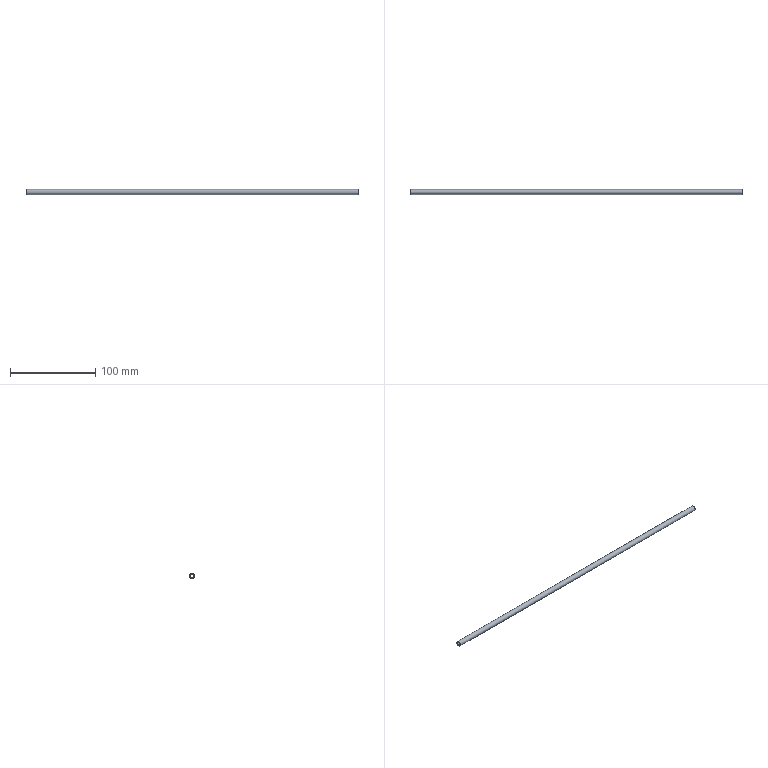Part | NX | features solid 2 | 1 solid | 4 faces | box 390 x 6 x 6 mm | volume 6126 mm3 | cylinder 2 | plane 2 | commonest cylinder face diameters 4 x1 6 x1
STEP:
#1=CARTESIAN_POINT('',(520.,-60.,347.));
#2=VERTEX_POINT('',#1);
#3=CARTESIAN_POINT('',(520.,-58.,347.));
#4=DIRECTION('',(-1.,0.,0.));
#5=DIRECTION('',(0.,-1.,0.));
#6=AXIS2_PLACEMENT_3D('',#3,#4,#5);
#7=CIRCLE('',#6,2.);
#8=EDGE_CURVE('',#2,#2,#7,.T.);
#9=ORIENTED_EDGE('',*,*,#8,.F.);
#10=EDGE_LOOP('',(#9));
#11=FACE_BOUND('',#10,.T.);
#12=CARTESIAN_POINT('',(130.,-60.,347.));
#13=VERTEX_POINT('',#12);
#14=CARTESIAN_POINT('',(130.,-58.,347.));
#15=DIRECTION('',(-1.,0.,0.));
#16=DIRECTION('',(0.,-1.,0.));
#17=AXIS2_PLACEMENT_3D('',#14,#15,#16);
#18=CIRCLE('',#17,2.);
#19=EDGE_CURVE('',#13,#13,#18,.T.);
#20=ORIENTED_EDGE('',*,*,#19,.T.);
#21=EDGE_LOOP('',(#20));
#22=FACE_BOUND('',#21,.T.);
#23=CARTESIAN_POINT('',(241.176,-58.,347.));
#24=DIRECTION('',(1.,0.,0.));
#25=DIRECTION('',(0.,1.,0.));
#26=AXIS2_PLACEMENT_3D('',#23,#24,#25);
#27=CYLINDRICAL_SURFACE('',#26,2.);
#28=ADVANCED_FACE('',(#11,#22),#27,.F.);
#29=CARTESIAN_POINT('',(520.,-61.,347.));
#30=VERTEX_POINT('',#29);
#31=CARTESIAN_POINT('',(520.,-58.,347.));
#32=DIRECTION('',(-1.,0.,0.));
#33=DIRECTION('',(0.,-1.,0.));
#34=AXIS2_PLACEMENT_3D('',#31,#32,#33);
#35=CIRCLE('',#34,3.);
#36=EDGE_CURVE('',#30,#30,#35,.T.);
#37=ORIENTED_EDGE('',*,*,#36,.T.);
#38=EDGE_LOOP('',(#37));
#39=FACE_BOUND('',#38,.T.);
#40=CARTESIAN_POINT('',(130.,-61.,347.));
#41=VERTEX_POINT('',#40);
#42=CARTESIAN_POINT('',(130.,-58.,347.));
#43=DIRECTION('',(-1.,0.,0.));
#44=DIRECTION('',(0.,-1.,0.));
#45=AXIS2_PLACEMENT_3D('',#42,#43,#44);
#46=CIRCLE('',#45,3.);
#47=EDGE_CURVE('',#41,#41,#46,.T.);
#48=ORIENTED_EDGE('',*,*,#47,.F.);
#49=EDGE_LOOP('',(#48));
#50=FACE_BOUND('',#49,.T.);
#51=CARTESIAN_POINT('',(241.176,-58.,347.));
#52=DIRECTION('',(1.,0.,0.));
#53=DIRECTION('',(0.,1.,0.));
#54=AXIS2_PLACEMENT_3D('',#51,#52,#53);
#55=CYLINDRICAL_SURFACE('',#54,3.);
#56=ADVANCED_FACE('',(#39,#50),#55,.T.);
#57=ORIENTED_EDGE('',*,*,#8,.T.);
#58=EDGE_LOOP('',(#57));
#59=FACE_BOUND('',#58,.T.);
#60=ORIENTED_EDGE('',*,*,#36,.F.);
#61=EDGE_LOOP('',(#60));
#62=FACE_BOUND('',#61,.T.);
#63=CARTESIAN_POINT('',(520.,-58.,347.));
#64=DIRECTION('',(-1.,0.,0.));
#65=DIRECTION('',(0.,-1.,0.));
#66=AXIS2_PLACEMENT_3D('',#63,#64,#65);
#67=PLANE('',#66);
#68=ADVANCED_FACE('',(#59,#62),#67,.F.);
#69=ORIENTED_EDGE('',*,*,#19,.F.);
#70=EDGE_LOOP('',(#69));
#71=FACE_BOUND('',#70,.T.);
#72=ORIENTED_EDGE('',*,*,#47,.T.);
#73=EDGE_LOOP('',(#72));
#74=FACE_BOUND('',#73,.T.);
#75=CARTESIAN_POINT('',(130.,35.,347.));
#76=DIRECTION('',(-1.,0.,0.));
#77=DIRECTION('',(0.,-1.,0.));
#78=AXIS2_PLACEMENT_3D('',#75,#76,#77);
#79=PLANE('',#78);
#80=ADVANCED_FACE('',(#71,#74),#79,.T.);
#81=CLOSED_SHELL('',(#28,#56,#68,#80));
#82=MANIFOLD_SOLID_BREP('',#81);
#83=(LENGTH_UNIT()NAMED_UNIT(*)SI_UNIT(.MILLI.,.METRE.));
#84=UNCERTAINTY_MEASURE_WITH_UNIT(LENGTH_MEASURE(0.00001),#83,'','');
#85=(NAMED_UNIT(*)PLANE_ANGLE_UNIT()SI_UNIT($,.RADIAN.));
#86=(NAMED_UNIT(*)SI_UNIT($,.STERADIAN.)SOLID_ANGLE_UNIT());
#87=(GEOMETRIC_REPRESENTATION_CONTEXT(3)GLOBAL_UNCERTAINTY_ASSIGNED_CONTEXT((#84))GLOBAL_UNIT_ASSIGNED_CONTEXT((#83,#85,#86))REPRESENTATION_CONTEXT('',''));
#88=ADVANCED_BREP_SHAPE_REPRESENTATION('',(#82),#87);